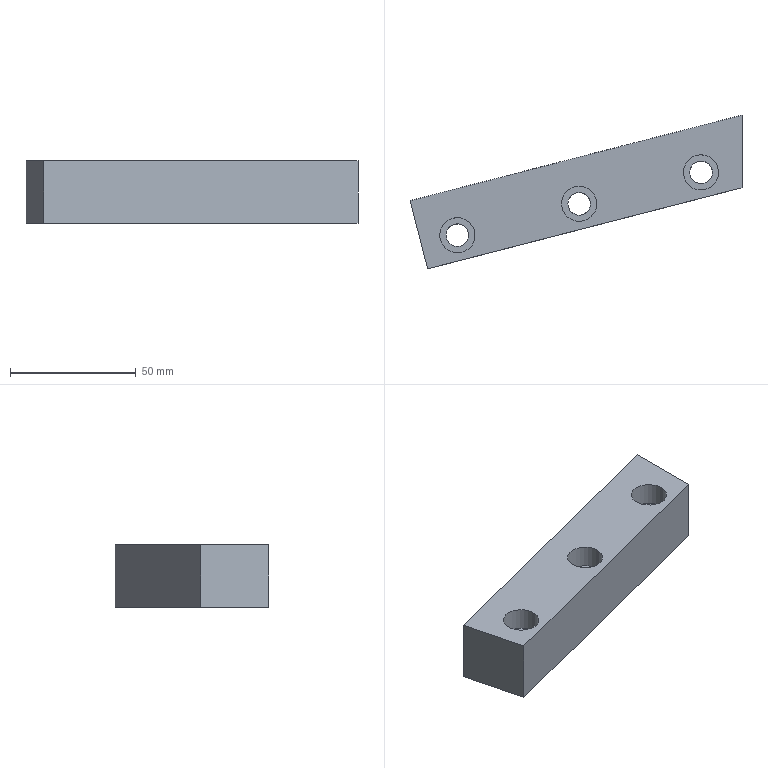Part | STEP file | 车灯-后视镜_id126_x_t | 1 solid | 15 faces | box 131.992 x 61.149 x 25 mm | volume 85679 mm3 | plane 9 | cylinder 6 | commonest cylinder face diameters 9 x3 14 x3
STEP:
#1=CARTESIAN_POINT('',(-256.992,-41.016,-25.286));
#2=VERTEX_POINT('',#1);
#3=CARTESIAN_POINT('',(-250.,-68.129,-25.286));
#4=VERTEX_POINT('',#3);
#5=CARTESIAN_POINT('',(-256.992,-41.016,-25.286));
#6=DIRECTION('',(0.2497,-0.9683,0.));
#7=VECTOR('',#6,1.);
#8=LINE('',#5,#7);
#9=EDGE_CURVE('',#2,#4,#8,.T.);
#10=ORIENTED_EDGE('',*,*,#9,.T.);
#11=CARTESIAN_POINT('',(-250.,-68.129,-0.2856));
#12=VERTEX_POINT('',#11);
#13=CARTESIAN_POINT('',(-250.,-68.129,-25.286));
#14=DIRECTION('',(0.,0.,1.));
#15=VECTOR('',#14,1.);
#16=LINE('',#13,#15);
#17=EDGE_CURVE('',#4,#12,#16,.T.);
#18=ORIENTED_EDGE('',*,*,#17,.T.);
#19=CARTESIAN_POINT('',(-256.992,-41.016,-0.2856));
#20=VERTEX_POINT('',#19);
#21=CARTESIAN_POINT('',(-256.992,-41.016,-0.2856));
#22=DIRECTION('',(-0.2497,0.9683,0.));
#23=VECTOR('',#22,1.);
#24=LINE('',#21,#23);
#25=EDGE_CURVE('',#12,#20,#24,.T.);
#26=ORIENTED_EDGE('',*,*,#25,.T.);
#27=CARTESIAN_POINT('',(-256.992,-41.016,-25.286));
#28=DIRECTION('',(0.,0.,1.));
#29=VECTOR('',#28,1.);
#30=LINE('',#27,#29);
#31=EDGE_CURVE('',#2,#20,#30,.T.);
#32=ORIENTED_EDGE('',*,*,#31,.F.);
#33=EDGE_LOOP('',(#10,#18,#26,#32));
#34=FACE_OUTER_BOUND('',#33,.T.);
#35=CARTESIAN_POINT('',(-250.,-68.129,-0.5));
#36=DIRECTION('',(-0.9683,-0.2497,0.));
#37=DIRECTION('',(0.2497,-0.9683,0.));
#38=AXIS2_PLACEMENT_3D('',#35,#36,#37);
#39=PLANE('',#38);
#40=ADVANCED_FACE('',(#34),#39,.T.);
#41=CARTESIAN_POINT('',(-125.,-6.98,-25.286));
#42=VERTEX_POINT('',#41);
#43=CARTESIAN_POINT('',(-125.,-35.896,-25.286));
#44=VERTEX_POINT('',#43);
#45=CARTESIAN_POINT('',(-125.,3.59,-25.286));
#46=DIRECTION('',(0.,-1.,0.));
#47=VECTOR('',#46,1.);
#48=LINE('',#45,#47);
#49=EDGE_CURVE('',#42,#44,#48,.T.);
#50=ORIENTED_EDGE('',*,*,#49,.F.);
#51=CARTESIAN_POINT('',(-125.,-6.98,-0.2856));
#52=VERTEX_POINT('',#51);
#53=CARTESIAN_POINT('',(-125.,-6.98,-25.286));
#54=DIRECTION('',(0.,0.,1.));
#55=VECTOR('',#54,1.);
#56=LINE('',#53,#55);
#57=EDGE_CURVE('',#42,#52,#56,.T.);
#58=ORIENTED_EDGE('',*,*,#57,.T.);
#59=CARTESIAN_POINT('',(-125.,-35.896,-0.2856));
#60=VERTEX_POINT('',#59);
#61=CARTESIAN_POINT('',(-125.,3.59,-0.2856));
#62=DIRECTION('',(0.,1.,0.));
#63=VECTOR('',#62,1.);
#64=LINE('',#61,#63);
#65=EDGE_CURVE('',#60,#52,#64,.T.);
#66=ORIENTED_EDGE('',*,*,#65,.F.);
#67=CARTESIAN_POINT('',(-125.,-35.896,-25.286));
#68=DIRECTION('',(0.,0.,1.));
#69=VECTOR('',#68,1.);
#70=LINE('',#67,#69);
#71=EDGE_CURVE('',#44,#60,#70,.T.);
#72=ORIENTED_EDGE('',*,*,#71,.F.);
#73=EDGE_LOOP('',(#50,#58,#66,#72));
#74=FACE_OUTER_BOUND('',#73,.T.);
#75=CARTESIAN_POINT('',(-125.,-90.701,-0.5));
#76=DIRECTION('',(-1.,0.,0.));
#77=DIRECTION('',(0.,-1.,0.));
#78=AXIS2_PLACEMENT_3D('',#75,#76,#77);
#79=PLANE('',#78);
#80=ADVANCED_FACE('',(#74),#79,.F.);
#81=CARTESIAN_POINT('',(-84.01,3.59,-25.286));
#82=DIRECTION('',(-0.9683,-0.2497,0.));
#83=VECTOR('',#82,1.);
#84=LINE('',#81,#83);
#85=EDGE_CURVE('',#42,#2,#84,.T.);
#86=ORIENTED_EDGE('',*,*,#85,.T.);
#87=ORIENTED_EDGE('',*,*,#31,.T.);
#88=CARTESIAN_POINT('',(-84.01,3.59,-0.2856));
#89=DIRECTION('',(-0.9683,-0.2497,0.));
#90=VECTOR('',#89,1.);
#91=LINE('',#88,#90);
#92=EDGE_CURVE('',#52,#20,#91,.T.);
#93=ORIENTED_EDGE('',*,*,#92,.F.);
#94=ORIENTED_EDGE('',*,*,#57,.F.);
#95=EDGE_LOOP('',(#86,#87,#93,#94));
#96=FACE_OUTER_BOUND('',#95,.T.);
#97=CARTESIAN_POINT('',(-84.01,3.59,-25.286));
#98=DIRECTION('',(-0.2497,0.9683,0.));
#99=DIRECTION('',(-0.9683,-0.2497,0.));
#100=AXIS2_PLACEMENT_3D('',#97,#98,#99);
#101=PLANE('',#100);
#102=ADVANCED_FACE('',(#96),#101,.T.);
#103=ORIENTED_EDGE('',*,*,#17,.F.);
#104=CARTESIAN_POINT('',(-77.018,-23.523,-25.286));
#105=DIRECTION('',(-0.9683,-0.2497,0.));
#106=VECTOR('',#105,1.);
#107=LINE('',#104,#106);
#108=EDGE_CURVE('',#44,#4,#107,.T.);
#109=ORIENTED_EDGE('',*,*,#108,.F.);
#110=ORIENTED_EDGE('',*,*,#71,.T.);
#111=CARTESIAN_POINT('',(-77.018,-23.523,-0.2856));
#112=DIRECTION('',(-0.9683,-0.2497,0.));
#113=VECTOR('',#112,1.);
#114=LINE('',#111,#113);
#115=EDGE_CURVE('',#60,#12,#114,.T.);
#116=ORIENTED_EDGE('',*,*,#115,.T.);
#117=EDGE_LOOP('',(#103,#109,#110,#116));
#118=FACE_OUTER_BOUND('',#117,.T.);
#119=CARTESIAN_POINT('',(-77.018,-23.523,-25.286));
#120=DIRECTION('',(-0.2497,0.9683,0.));
#121=DIRECTION('',(-0.9683,-0.2497,0.));
#122=AXIS2_PLACEMENT_3D('',#119,#120,#121);
#123=PLANE('',#122);
#124=ADVANCED_FACE('',(#118),#123,.F.);
#125=CARTESIAN_POINT('',(-236.379,-61.518,-0.2856));
#126=VERTEX_POINT('',#125);
#127=CARTESIAN_POINT('',(-238.127,-54.74,-0.2856));
#128=DIRECTION('',(0.,0.,-1.));
#129=DIRECTION('',(0.2497,-0.9683,0.));
#130=AXIS2_PLACEMENT_3D('',#127,#128,#129);
#131=CIRCLE('',#130,7.);
#132=EDGE_CURVE('',#126,#126,#131,.T.);
#133=ORIENTED_EDGE('',*,*,#132,.T.);
#134=EDGE_LOOP('',(#133));
#135=FACE_BOUND('',#134,.T.);
#136=CARTESIAN_POINT('',(-187.963,-49.033,-0.2856));
#137=VERTEX_POINT('',#136);
#138=CARTESIAN_POINT('',(-189.711,-42.255,-0.2856));
#139=DIRECTION('',(0.,0.,-1.));
#140=DIRECTION('',(0.2497,-0.9683,0.));
#141=AXIS2_PLACEMENT_3D('',#138,#139,#140);
#142=CIRCLE('',#141,7.);
#143=EDGE_CURVE('',#137,#137,#142,.T.);
#144=ORIENTED_EDGE('',*,*,#143,.T.);
#145=EDGE_LOOP('',(#144));
#146=FACE_BOUND('',#145,.T.);
#147=CARTESIAN_POINT('',(-139.547,-36.548,-0.2856));
#148=VERTEX_POINT('',#147);
#149=CARTESIAN_POINT('',(-141.294,-29.77,-0.2856));
#150=DIRECTION('',(0.,0.,-1.));
#151=DIRECTION('',(0.2497,-0.9683,0.));
#152=AXIS2_PLACEMENT_3D('',#149,#150,#151);
#153=CIRCLE('',#152,7.);
#154=EDGE_CURVE('',#148,#148,#153,.T.);
#155=ORIENTED_EDGE('',*,*,#154,.T.);
#156=EDGE_LOOP('',(#155));
#157=FACE_BOUND('',#156,.T.);
#158=ORIENTED_EDGE('',*,*,#25,.F.);
#159=ORIENTED_EDGE('',*,*,#115,.F.);
#160=ORIENTED_EDGE('',*,*,#65,.T.);
#161=ORIENTED_EDGE('',*,*,#92,.T.);
#162=EDGE_LOOP('',(#158,#159,#160,#161));
#163=FACE_BOUND('',#162,.T.);
#164=CARTESIAN_POINT('',(-84.01,3.59,-0.2856));
#165=DIRECTION('',(0.,0.,-1.));
#166=DIRECTION('',(-0.9683,-0.2497,0.));
#167=AXIS2_PLACEMENT_3D('',#164,#165,#166);
#168=PLANE('',#167);
#169=ADVANCED_FACE('',(#135,#146,#157,#163),#168,.F.);
#170=CARTESIAN_POINT('',(-237.003,-59.098,-25.286));
#171=VERTEX_POINT('',#170);
#172=CARTESIAN_POINT('',(-238.127,-54.74,-25.286));
#173=DIRECTION('',(0.,0.,1.));
#174=DIRECTION('',(0.2497,-0.9683,0.));
#175=AXIS2_PLACEMENT_3D('',#172,#173,#174);
#176=CIRCLE('',#175,4.5);
#177=EDGE_CURVE('',#171,#171,#176,.T.);
#178=ORIENTED_EDGE('',*,*,#177,.T.);
#179=EDGE_LOOP('',(#178));
#180=FACE_BOUND('',#179,.T.);
#181=CARTESIAN_POINT('',(-188.587,-46.613,-25.286));
#182=VERTEX_POINT('',#181);
#183=CARTESIAN_POINT('',(-189.711,-42.255,-25.286));
#184=DIRECTION('',(0.,0.,1.));
#185=DIRECTION('',(0.2497,-0.9683,0.));
#186=AXIS2_PLACEMENT_3D('',#183,#184,#185);
#187=CIRCLE('',#186,4.5);
#188=EDGE_CURVE('',#182,#182,#187,.T.);
#189=ORIENTED_EDGE('',*,*,#188,.T.);
#190=EDGE_LOOP('',(#189));
#191=FACE_BOUND('',#190,.T.);
#192=CARTESIAN_POINT('',(-140.171,-34.128,-25.286));
#193=VERTEX_POINT('',#192);
#194=CARTESIAN_POINT('',(-141.294,-29.77,-25.286));
#195=DIRECTION('',(0.,0.,1.));
#196=DIRECTION('',(0.2497,-0.9683,0.));
#197=AXIS2_PLACEMENT_3D('',#194,#195,#196);
#198=CIRCLE('',#197,4.5);
#199=EDGE_CURVE('',#193,#193,#198,.T.);
#200=ORIENTED_EDGE('',*,*,#199,.T.);
#201=EDGE_LOOP('',(#200));
#202=FACE_BOUND('',#201,.T.);
#203=ORIENTED_EDGE('',*,*,#9,.F.);
#204=ORIENTED_EDGE('',*,*,#85,.F.);
#205=ORIENTED_EDGE('',*,*,#49,.T.);
#206=ORIENTED_EDGE('',*,*,#108,.T.);
#207=EDGE_LOOP('',(#203,#204,#205,#206));
#208=FACE_BOUND('',#207,.T.);
#209=CARTESIAN_POINT('',(-84.01,3.59,-25.286));
#210=DIRECTION('',(0.,0.,-1.));
#211=DIRECTION('',(-0.9683,-0.2497,0.));
#212=AXIS2_PLACEMENT_3D('',#209,#210,#211);
#213=PLANE('',#212);
#214=ADVANCED_FACE('',(#180,#191,#202,#208),#213,.T.);
#215=CARTESIAN_POINT('',(-145.794,-29.77,-9.286));
#216=VERTEX_POINT('',#215);
#217=CARTESIAN_POINT('',(-141.294,-29.77,-9.286));
#218=DIRECTION('',(0.,0.,1.));
#219=DIRECTION('',(-1.,0.,0.));
#220=AXIS2_PLACEMENT_3D('',#217,#218,#219);
#221=CIRCLE('',#220,4.5);
#222=EDGE_CURVE('',#216,#216,#221,.T.);
#223=ORIENTED_EDGE('',*,*,#222,.T.);
#224=EDGE_LOOP('',(#223));
#225=FACE_BOUND('',#224,.T.);
#226=ORIENTED_EDGE('',*,*,#199,.F.);
#227=EDGE_LOOP('',(#226));
#228=FACE_BOUND('',#227,.T.);
#229=CARTESIAN_POINT('',(-141.294,-29.77,-24.786));
#230=DIRECTION('',(0.,0.,1.));
#231=DIRECTION('',(-0.2497,0.9683,0.));
#232=AXIS2_PLACEMENT_3D('',#229,#230,#231);
#233=CYLINDRICAL_SURFACE('',#232,4.5);
#234=ADVANCED_FACE('',(#225,#228),#233,.F.);
#235=ORIENTED_EDGE('',*,*,#222,.F.);
#236=EDGE_LOOP('',(#235));
#237=FACE_BOUND('',#236,.T.);
#238=CARTESIAN_POINT('',(-143.042,-22.992,-9.286));
#239=VERTEX_POINT('',#238);
#240=CARTESIAN_POINT('',(-141.294,-29.77,-9.286));
#241=DIRECTION('',(0.,0.,1.));
#242=DIRECTION('',(-0.2497,0.9683,0.));
#243=AXIS2_PLACEMENT_3D('',#240,#241,#242);
#244=CIRCLE('',#243,7.);
#245=EDGE_CURVE('',#239,#239,#244,.T.);
#246=ORIENTED_EDGE('',*,*,#245,.T.);
#247=EDGE_LOOP('',(#246));
#248=FACE_BOUND('',#247,.T.);
#249=CARTESIAN_POINT('',(-141.294,-29.77,-9.286));
#250=DIRECTION('',(0.,0.,-1.));
#251=DIRECTION('',(0.2497,-0.9683,0.));
#252=AXIS2_PLACEMENT_3D('',#249,#250,#251);
#253=PLANE('',#252);
#254=ADVANCED_FACE('',(#237,#248),#253,.F.);
#255=ORIENTED_EDGE('',*,*,#245,.F.);
#256=EDGE_LOOP('',(#255));
#257=FACE_BOUND('',#256,.T.);
#258=ORIENTED_EDGE('',*,*,#154,.F.);
#259=EDGE_LOOP('',(#258));
#260=FACE_BOUND('',#259,.T.);
#261=CARTESIAN_POINT('',(-141.294,-29.77,-0.2856));
#262=DIRECTION('',(0.,0.,-1.));
#263=DIRECTION('',(0.2497,-0.9683,0.));
#264=AXIS2_PLACEMENT_3D('',#261,#262,#263);
#265=CYLINDRICAL_SURFACE('',#264,7.);
#266=ADVANCED_FACE('',(#257,#260),#265,.F.);
#267=CARTESIAN_POINT('',(-194.211,-42.255,-9.286));
#268=VERTEX_POINT('',#267);
#269=CARTESIAN_POINT('',(-189.711,-42.255,-9.286));
#270=DIRECTION('',(0.,0.,1.));
#271=DIRECTION('',(-1.,0.,0.));
#272=AXIS2_PLACEMENT_3D('',#269,#270,#271);
#273=CIRCLE('',#272,4.5);
#274=EDGE_CURVE('',#268,#268,#273,.T.);
#275=ORIENTED_EDGE('',*,*,#274,.T.);
#276=EDGE_LOOP('',(#275));
#277=FACE_BOUND('',#276,.T.);
#278=ORIENTED_EDGE('',*,*,#188,.F.);
#279=EDGE_LOOP('',(#278));
#280=FACE_BOUND('',#279,.T.);
#281=CARTESIAN_POINT('',(-189.711,-42.255,-24.786));
#282=DIRECTION('',(0.,0.,1.));
#283=DIRECTION('',(-0.2497,0.9683,0.));
#284=AXIS2_PLACEMENT_3D('',#281,#282,#283);
#285=CYLINDRICAL_SURFACE('',#284,4.5);
#286=ADVANCED_FACE('',(#277,#280),#285,.F.);
#287=ORIENTED_EDGE('',*,*,#274,.F.);
#288=EDGE_LOOP('',(#287));
#289=FACE_BOUND('',#288,.T.);
#290=CARTESIAN_POINT('',(-191.458,-35.477,-9.286));
#291=VERTEX_POINT('',#290);
#292=CARTESIAN_POINT('',(-189.711,-42.255,-9.286));
#293=DIRECTION('',(0.,0.,1.));
#294=DIRECTION('',(-0.2497,0.9683,0.));
#295=AXIS2_PLACEMENT_3D('',#292,#293,#294);
#296=CIRCLE('',#295,7.);
#297=EDGE_CURVE('',#291,#291,#296,.T.);
#298=ORIENTED_EDGE('',*,*,#297,.T.);
#299=EDGE_LOOP('',(#298));
#300=FACE_BOUND('',#299,.T.);
#301=CARTESIAN_POINT('',(-189.711,-42.255,-9.286));
#302=DIRECTION('',(0.,0.,-1.));
#303=DIRECTION('',(0.2497,-0.9683,0.));
#304=AXIS2_PLACEMENT_3D('',#301,#302,#303);
#305=PLANE('',#304);
#306=ADVANCED_FACE('',(#289,#300),#305,.F.);
#307=ORIENTED_EDGE('',*,*,#297,.F.);
#308=EDGE_LOOP('',(#307));
#309=FACE_BOUND('',#308,.T.);
#310=ORIENTED_EDGE('',*,*,#143,.F.);
#311=EDGE_LOOP('',(#310));
#312=FACE_BOUND('',#311,.T.);
#313=CARTESIAN_POINT('',(-189.711,-42.255,-0.2856));
#314=DIRECTION('',(0.,0.,-1.));
#315=DIRECTION('',(0.2497,-0.9683,0.));
#316=AXIS2_PLACEMENT_3D('',#313,#314,#315);
#317=CYLINDRICAL_SURFACE('',#316,7.);
#318=ADVANCED_FACE('',(#309,#312),#317,.F.);
#319=CARTESIAN_POINT('',(-242.627,-54.74,-9.286));
#320=VERTEX_POINT('',#319);
#321=CARTESIAN_POINT('',(-238.127,-54.74,-9.286));
#322=DIRECTION('',(0.,0.,1.));
#323=DIRECTION('',(-1.,0.,0.));
#324=AXIS2_PLACEMENT_3D('',#321,#322,#323);
#325=CIRCLE('',#324,4.5);
#326=EDGE_CURVE('',#320,#320,#325,.T.);
#327=ORIENTED_EDGE('',*,*,#326,.T.);
#328=EDGE_LOOP('',(#327));
#329=FACE_BOUND('',#328,.T.);
#330=ORIENTED_EDGE('',*,*,#177,.F.);
#331=EDGE_LOOP('',(#330));
#332=FACE_BOUND('',#331,.T.);
#333=CARTESIAN_POINT('',(-238.127,-54.74,-24.786));
#334=DIRECTION('',(0.,0.,1.));
#335=DIRECTION('',(-0.2497,0.9683,0.));
#336=AXIS2_PLACEMENT_3D('',#333,#334,#335);
#337=CYLINDRICAL_SURFACE('',#336,4.5);
#338=ADVANCED_FACE('',(#329,#332),#337,.F.);
#339=ORIENTED_EDGE('',*,*,#326,.F.);
#340=EDGE_LOOP('',(#339));
#341=FACE_BOUND('',#340,.T.);
#342=CARTESIAN_POINT('',(-239.875,-47.962,-9.286));
#343=VERTEX_POINT('',#342);
#344=CARTESIAN_POINT('',(-238.127,-54.74,-9.286));
#345=DIRECTION('',(0.,0.,1.));
#346=DIRECTION('',(-0.2497,0.9683,0.));
#347=AXIS2_PLACEMENT_3D('',#344,#345,#346);
#348=CIRCLE('',#347,7.);
#349=EDGE_CURVE('',#343,#343,#348,.T.);
#350=ORIENTED_EDGE('',*,*,#349,.T.);
#351=EDGE_LOOP('',(#350));
#352=FACE_BOUND('',#351,.T.);
#353=CARTESIAN_POINT('',(-238.127,-54.74,-9.286));
#354=DIRECTION('',(0.,0.,-1.));
#355=DIRECTION('',(0.2497,-0.9683,0.));
#356=AXIS2_PLACEMENT_3D('',#353,#354,#355);
#357=PLANE('',#356);
#358=ADVANCED_FACE('',(#341,#352),#357,.F.);
#359=ORIENTED_EDGE('',*,*,#349,.F.);
#360=EDGE_LOOP('',(#359));
#361=FACE_BOUND('',#360,.T.);
#362=ORIENTED_EDGE('',*,*,#132,.F.);
#363=EDGE_LOOP('',(#362));
#364=FACE_BOUND('',#363,.T.);
#365=CARTESIAN_POINT('',(-238.127,-54.74,-0.2856));
#366=DIRECTION('',(0.,0.,-1.));
#367=DIRECTION('',(0.2497,-0.9683,0.));
#368=AXIS2_PLACEMENT_3D('',#365,#366,#367);
#369=CYLINDRICAL_SURFACE('',#368,7.);
#370=ADVANCED_FACE('',(#361,#364),#369,.F.);
#371=CLOSED_SHELL('',(#40,#80,#102,#124,#169,#214,#234,#254,#266,#286,#306,#318,#338,#358,#370));
#372=MANIFOLD_SOLID_BREP('',#371);
#373=(LENGTH_UNIT()NAMED_UNIT(*)SI_UNIT(.MILLI.,.METRE.));
#374=UNCERTAINTY_MEASURE_WITH_UNIT(LENGTH_MEASURE(0.00002),#373,'','');
#375=(NAMED_UNIT(*)PLANE_ANGLE_UNIT()SI_UNIT($,.RADIAN.));
#376=PLANE_ANGLE_MEASURE_WITH_UNIT(PLANE_ANGLE_MEASURE(0.01745),#375);
#377=DIMENSIONAL_EXPONENTS(0.,0.,0.,0.,0.,0.,0.);
#378=(CONVERSION_BASED_UNIT('DEGREE',#376)NAMED_UNIT(#377)PLANE_ANGLE_UNIT());
#379=(NAMED_UNIT(*)SI_UNIT($,.STERADIAN.)SOLID_ANGLE_UNIT());
#380=(GEOMETRIC_REPRESENTATION_CONTEXT(3)GLOBAL_UNCERTAINTY_ASSIGNED_CONTEXT((#374))GLOBAL_UNIT_ASSIGNED_CONTEXT((#373,#378,#379))REPRESENTATION_CONTEXT('',''));
#381=ADVANCED_BREP_SHAPE_REPRESENTATION('',(#372),#380);